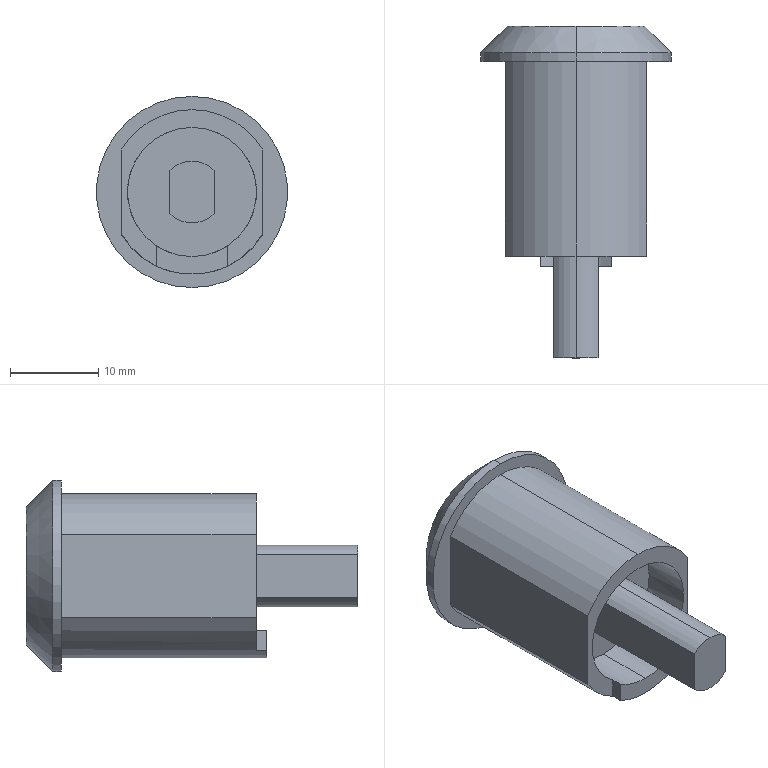Part | SolidWorks | features BaseBody 1 | 1 solid | 36 faces | box 21.6 x 37.5 x 21.6 mm | volume 6258 mm3 | plane 20 | cylinder 14 | cone 2 | commonest cylinder face diameters 7 x5 18.6 x3 10 x2 14.6 x2 21.6 x2
STEP:
#1=CARTESIAN_POINT('',(0.,-33.5,3.5));
#2=VERTEX_POINT('',#1);
#3=CARTESIAN_POINT('',(-2.5,-33.5,2.449));
#4=VERTEX_POINT('',#3);
#5=CARTESIAN_POINT('',(0.,-33.5,0.));
#6=DIRECTION('',(0.,-1.,0.));
#7=DIRECTION('',(0.,0.,1.));
#8=AXIS2_PLACEMENT_3D('',#5,#6,#7);
#9=CIRCLE('',#8,3.5);
#10=EDGE_CURVE('',#2,#4,#9,.T.);
#11=ORIENTED_EDGE('',*,*,#10,.F.);
#12=CARTESIAN_POINT('',(0.,-16.5,3.5));
#13=VERTEX_POINT('',#12);
#14=CARTESIAN_POINT('',(0.,-33.5,3.5));
#15=DIRECTION('',(0.,1.,0.));
#16=VECTOR('',#15,1000.);
#17=LINE('',#14,#16);
#18=EDGE_CURVE('',#2,#13,#17,.T.);
#19=ORIENTED_EDGE('',*,*,#18,.T.);
#20=CARTESIAN_POINT('',(-2.5,-16.5,2.449));
#21=VERTEX_POINT('',#20);
#22=CARTESIAN_POINT('',(0.,-16.5,0.));
#23=DIRECTION('',(0.,1.,0.));
#24=DIRECTION('',(0.,0.,1.));
#25=AXIS2_PLACEMENT_3D('',#22,#23,#24);
#26=CIRCLE('',#25,3.5);
#27=EDGE_CURVE('',#21,#13,#26,.T.);
#28=ORIENTED_EDGE('',*,*,#27,.F.);
#29=CARTESIAN_POINT('',(-2.5,-25.,2.449));
#30=DIRECTION('',(0.,1.,0.));
#31=VECTOR('',#30,1000.);
#32=LINE('',#29,#31);
#33=EDGE_CURVE('',#4,#21,#32,.T.);
#34=ORIENTED_EDGE('',*,*,#33,.F.);
#35=EDGE_LOOP('',(#11,#19,#28,#34));
#36=FACE_OUTER_BOUND('',#35,.T.);
#37=CARTESIAN_POINT('',(0.,-33.5,0.));
#38=DIRECTION('',(0.,1.,0.));
#39=DIRECTION('',(0.,0.,1.));
#40=AXIS2_PLACEMENT_3D('',#37,#38,#39);
#41=CYLINDRICAL_SURFACE('',#40,3.5);
#42=ADVANCED_FACE('',(#36),#41,.T.);
#43=CARTESIAN_POINT('',(0.,-16.5,7.3));
#44=VERTEX_POINT('',#43);
#45=CARTESIAN_POINT('',(0.,-16.5,-7.3));
#46=VERTEX_POINT('',#45);
#47=CARTESIAN_POINT('',(0.,-16.5,0.));
#48=DIRECTION('',(0.,-1.,0.));
#49=DIRECTION('',(0.,0.,-1.));
#50=AXIS2_PLACEMENT_3D('',#47,#48,#49);
#51=CIRCLE('',#50,7.3);
#52=EDGE_CURVE('',#44,#46,#51,.T.);
#53=ORIENTED_EDGE('',*,*,#52,.F.);
#54=CARTESIAN_POINT('',(0.,-22.,7.3));
#55=VERTEX_POINT('',#54);
#56=CARTESIAN_POINT('',(0.,-16.5,7.3));
#57=DIRECTION('',(0.,-1.,0.));
#58=VECTOR('',#57,1000.);
#59=LINE('',#56,#58);
#60=EDGE_CURVE('',#44,#55,#59,.T.);
#61=ORIENTED_EDGE('',*,*,#60,.T.);
#62=CARTESIAN_POINT('',(-4.,-22.,-6.107));
#63=VERTEX_POINT('',#62);
#64=CARTESIAN_POINT('',(0.,-22.,0.));
#65=DIRECTION('',(0.,-1.,0.));
#66=DIRECTION('',(0.,0.,-1.));
#67=AXIS2_PLACEMENT_3D('',#64,#65,#66);
#68=CIRCLE('',#67,7.3);
#69=EDGE_CURVE('',#55,#63,#68,.T.);
#70=ORIENTED_EDGE('',*,*,#69,.T.);
#71=CARTESIAN_POINT('',(-4.,-23.2,-6.107));
#72=VERTEX_POINT('',#71);
#73=CARTESIAN_POINT('',(-4.,-22.6,-6.107));
#74=DIRECTION('',(0.,-1.,0.));
#75=VECTOR('',#74,1000.);
#76=LINE('',#73,#75);
#77=EDGE_CURVE('',#63,#72,#76,.T.);
#78=ORIENTED_EDGE('',*,*,#77,.T.);
#79=CARTESIAN_POINT('',(0.,-23.2,-7.3));
#80=VERTEX_POINT('',#79);
#81=CARTESIAN_POINT('',(0.,-23.2,0.));
#82=DIRECTION('',(0.,-1.,0.));
#83=DIRECTION('',(0.,0.,-1.));
#84=AXIS2_PLACEMENT_3D('',#81,#82,#83);
#85=CIRCLE('',#84,7.3);
#86=EDGE_CURVE('',#72,#80,#85,.T.);
#87=ORIENTED_EDGE('',*,*,#86,.T.);
#88=CARTESIAN_POINT('',(0.,-16.5,-7.3));
#89=DIRECTION('',(0.,-1.,0.));
#90=VECTOR('',#89,1000.);
#91=LINE('',#88,#90);
#92=EDGE_CURVE('',#46,#80,#91,.T.);
#93=ORIENTED_EDGE('',*,*,#92,.F.);
#94=EDGE_LOOP('',(#53,#61,#70,#78,#87,#93));
#95=FACE_OUTER_BOUND('',#94,.T.);
#96=CARTESIAN_POINT('',(0.,-16.5,0.));
#97=DIRECTION('',(0.,-1.,0.));
#98=DIRECTION('',(0.,0.,-1.));
#99=AXIS2_PLACEMENT_3D('',#96,#97,#98);
#100=CYLINDRICAL_SURFACE('',#99,7.3);
#101=ADVANCED_FACE('',(#95),#100,.F.);
#102=CARTESIAN_POINT('',(0.,-22.,9.3));
#103=VERTEX_POINT('',#102);
#104=CARTESIAN_POINT('',(-8.,-22.,4.742));
#105=VERTEX_POINT('',#104);
#106=CARTESIAN_POINT('',(0.,-22.,0.));
#107=DIRECTION('',(0.,-1.,0.));
#108=DIRECTION('',(0.,0.,1.));
#109=AXIS2_PLACEMENT_3D('',#106,#107,#108);
#110=CIRCLE('',#109,9.3);
#111=EDGE_CURVE('',#103,#105,#110,.T.);
#112=ORIENTED_EDGE('',*,*,#111,.F.);
#113=CARTESIAN_POINT('',(0.,0.,9.3));
#114=VERTEX_POINT('',#113);
#115=CARTESIAN_POINT('',(0.,-22.,9.3));
#116=DIRECTION('',(0.,1.,0.));
#117=VECTOR('',#116,1000.);
#118=LINE('',#115,#117);
#119=EDGE_CURVE('',#103,#114,#118,.T.);
#120=ORIENTED_EDGE('',*,*,#119,.T.);
#121=CARTESIAN_POINT('',(-8.,0.,4.742));
#122=VERTEX_POINT('',#121);
#123=CARTESIAN_POINT('',(0.,0.,0.));
#124=DIRECTION('',(0.,1.,0.));
#125=DIRECTION('',(0.,0.,1.));
#126=AXIS2_PLACEMENT_3D('',#123,#124,#125);
#127=CIRCLE('',#126,9.3);
#128=EDGE_CURVE('',#122,#114,#127,.T.);
#129=ORIENTED_EDGE('',*,*,#128,.F.);
#130=CARTESIAN_POINT('',(-8.,-11.,4.742));
#131=DIRECTION('',(0.,-1.,0.));
#132=VECTOR('',#131,1000.);
#133=LINE('',#130,#132);
#134=EDGE_CURVE('',#122,#105,#133,.T.);
#135=ORIENTED_EDGE('',*,*,#134,.T.);
#136=EDGE_LOOP('',(#112,#120,#129,#135));
#137=FACE_OUTER_BOUND('',#136,.T.);
#138=CARTESIAN_POINT('',(0.,-22.,0.));
#139=DIRECTION('',(0.,1.,0.));
#140=DIRECTION('',(0.,0.,1.));
#141=AXIS2_PLACEMENT_3D('',#138,#139,#140);
#142=CYLINDRICAL_SURFACE('',#141,9.3);
#143=ADVANCED_FACE('',(#137),#142,.T.);
#144=CARTESIAN_POINT('',(0.,1.,10.8));
#145=VERTEX_POINT('',#144);
#146=CARTESIAN_POINT('',(0.,1.,-10.8));
#147=VERTEX_POINT('',#146);
#148=CARTESIAN_POINT('',(0.,1.,0.));
#149=DIRECTION('',(0.,1.,0.));
#150=DIRECTION('',(0.,0.,-1.));
#151=AXIS2_PLACEMENT_3D('',#148,#149,#150);
#152=CIRCLE('',#151,10.8);
#153=EDGE_CURVE('',#145,#147,#152,.T.);
#154=ORIENTED_EDGE('',*,*,#153,.F.);
#155=CARTESIAN_POINT('',(0.,0.,10.8));
#156=VERTEX_POINT('',#155);
#157=CARTESIAN_POINT('',(0.,1.,10.8));
#158=DIRECTION('',(0.,-1.,0.));
#159=VECTOR('',#158,1000.);
#160=LINE('',#157,#159);
#161=EDGE_CURVE('',#145,#156,#160,.T.);
#162=ORIENTED_EDGE('',*,*,#161,.T.);
#163=CARTESIAN_POINT('',(0.,0.,-10.8));
#164=VERTEX_POINT('',#163);
#165=CARTESIAN_POINT('',(0.,0.,0.));
#166=DIRECTION('',(0.,1.,0.));
#167=DIRECTION('',(0.,0.,-1.));
#168=AXIS2_PLACEMENT_3D('',#165,#166,#167);
#169=CIRCLE('',#168,10.8);
#170=EDGE_CURVE('',#156,#164,#169,.T.);
#171=ORIENTED_EDGE('',*,*,#170,.T.);
#172=CARTESIAN_POINT('',(0.,1.,-10.8));
#173=DIRECTION('',(0.,-1.,0.));
#174=VECTOR('',#173,1000.);
#175=LINE('',#172,#174);
#176=EDGE_CURVE('',#147,#164,#175,.T.);
#177=ORIENTED_EDGE('',*,*,#176,.F.);
#178=EDGE_LOOP('',(#154,#162,#171,#177));
#179=FACE_OUTER_BOUND('',#178,.T.);
#180=CARTESIAN_POINT('',(0.,1.,0.));
#181=DIRECTION('',(0.,-1.,0.));
#182=DIRECTION('',(0.,0.,-1.));
#183=AXIS2_PLACEMENT_3D('',#180,#181,#182);
#184=CYLINDRICAL_SURFACE('',#183,10.8);
#185=ADVANCED_FACE('',(#179),#184,.T.);
#186=CARTESIAN_POINT('',(0.,4.,7.8));
#187=VERTEX_POINT('',#186);
#188=CARTESIAN_POINT('',(0.,4.,-7.8));
#189=VERTEX_POINT('',#188);
#190=CARTESIAN_POINT('',(0.,4.,0.));
#191=DIRECTION('',(0.,1.,0.));
#192=DIRECTION('',(0.,0.,-1.));
#193=AXIS2_PLACEMENT_3D('',#190,#191,#192);
#194=CIRCLE('',#193,7.8);
#195=EDGE_CURVE('',#187,#189,#194,.T.);
#196=ORIENTED_EDGE('',*,*,#195,.F.);
#197=CARTESIAN_POINT('',(0.,4.,7.8));
#198=DIRECTION('',(0.,-0.7071,0.7071));
#199=VECTOR('',#198,1000.);
#200=LINE('',#197,#199);
#201=EDGE_CURVE('',#187,#145,#200,.T.);
#202=ORIENTED_EDGE('',*,*,#201,.T.);
#203=ORIENTED_EDGE('',*,*,#153,.T.);
#204=CARTESIAN_POINT('',(0.,4.,-7.8));
#205=DIRECTION('',(0.,-0.7071,-0.7071));
#206=VECTOR('',#205,1000.);
#207=LINE('',#204,#206);
#208=EDGE_CURVE('',#189,#147,#207,.T.);
#209=ORIENTED_EDGE('',*,*,#208,.F.);
#210=EDGE_LOOP('',(#196,#202,#203,#209));
#211=FACE_OUTER_BOUND('',#210,.T.);
#212=CARTESIAN_POINT('',(0.,4.,0.));
#213=DIRECTION('',(0.,-1.,0.));
#214=DIRECTION('',(0.,0.,-1.));
#215=AXIS2_PLACEMENT_3D('',#212,#213,#214);
#216=CONICAL_SURFACE('',#215,7.8,0.7854);
#217=ADVANCED_FACE('',(#211),#216,.T.);
#218=CARTESIAN_POINT('',(0.,4.,-5.));
#219=VERTEX_POINT('',#218);
#220=CARTESIAN_POINT('',(1.,4.,4.899));
#221=VERTEX_POINT('',#220);
#222=CARTESIAN_POINT('',(0.,4.,0.));
#223=DIRECTION('',(0.,-1.,0.));
#224=DIRECTION('',(0.,0.,-1.));
#225=AXIS2_PLACEMENT_3D('',#222,#223,#224);
#226=CIRCLE('',#225,5.);
#227=EDGE_CURVE('',#219,#221,#226,.T.);
#228=ORIENTED_EDGE('',*,*,#227,.F.);
#229=CARTESIAN_POINT('',(0.,0.,-5.));
#230=VERTEX_POINT('',#229);
#231=CARTESIAN_POINT('',(0.,4.,-5.));
#232=DIRECTION('',(0.,-1.,0.));
#233=VECTOR('',#232,1000.);
#234=LINE('',#231,#233);
#235=EDGE_CURVE('',#219,#230,#234,.T.);
#236=ORIENTED_EDGE('',*,*,#235,.T.);
#237=CARTESIAN_POINT('',(1.,0.,4.899));
#238=VERTEX_POINT('',#237);
#239=CARTESIAN_POINT('',(0.,0.,0.));
#240=DIRECTION('',(0.,-1.,0.));
#241=DIRECTION('',(0.,0.,-1.));
#242=AXIS2_PLACEMENT_3D('',#239,#240,#241);
#243=CIRCLE('',#242,5.);
#244=EDGE_CURVE('',#230,#238,#243,.T.);
#245=ORIENTED_EDGE('',*,*,#244,.T.);
#246=CARTESIAN_POINT('',(1.,2.,4.899));
#247=DIRECTION('',(0.,1.,0.));
#248=VECTOR('',#247,1000.);
#249=LINE('',#246,#248);
#250=EDGE_CURVE('',#238,#221,#249,.T.);
#251=ORIENTED_EDGE('',*,*,#250,.T.);
#252=EDGE_LOOP('',(#228,#236,#245,#251));
#253=FACE_OUTER_BOUND('',#252,.T.);
#254=CARTESIAN_POINT('',(0.,4.,0.));
#255=DIRECTION('',(0.,-1.,0.));
#256=DIRECTION('',(0.,0.,-1.));
#257=AXIS2_PLACEMENT_3D('',#254,#255,#256);
#258=CYLINDRICAL_SURFACE('',#257,5.);
#259=ADVANCED_FACE('',(#253),#258,.F.);
#260=CARTESIAN_POINT('',(0.,4.,-3.5));
#261=VERTEX_POINT('',#260);
#262=CARTESIAN_POINT('',(-1.,4.,3.354));
#263=VERTEX_POINT('',#262);
#264=CARTESIAN_POINT('',(0.,4.,0.));
#265=DIRECTION('',(0.,1.,0.));
#266=DIRECTION('',(0.,0.,-1.));
#267=AXIS2_PLACEMENT_3D('',#264,#265,#266);
#268=CIRCLE('',#267,3.5);
#269=EDGE_CURVE('',#261,#263,#268,.T.);
#270=ORIENTED_EDGE('',*,*,#269,.F.);
#271=CARTESIAN_POINT('',(0.,0.,-3.5));
#272=VERTEX_POINT('',#271);
#273=CARTESIAN_POINT('',(0.,4.,-3.5));
#274=DIRECTION('',(0.,-1.,0.));
#275=VECTOR('',#274,1000.);
#276=LINE('',#273,#275);
#277=EDGE_CURVE('',#261,#272,#276,.T.);
#278=ORIENTED_EDGE('',*,*,#277,.T.);
#279=CARTESIAN_POINT('',(-1.,0.,3.354));
#280=VERTEX_POINT('',#279);
#281=CARTESIAN_POINT('',(0.,0.,0.));
#282=DIRECTION('',(0.,1.,0.));
#283=DIRECTION('',(0.,0.,-1.));
#284=AXIS2_PLACEMENT_3D('',#281,#282,#283);
#285=CIRCLE('',#284,3.5);
#286=EDGE_CURVE('',#272,#280,#285,.T.);
#287=ORIENTED_EDGE('',*,*,#286,.T.);
#288=CARTESIAN_POINT('',(-1.,2.,3.354));
#289=DIRECTION('',(0.,-1.,0.));
#290=VECTOR('',#289,1000.);
#291=LINE('',#288,#290);
#292=EDGE_CURVE('',#263,#280,#291,.T.);
#293=ORIENTED_EDGE('',*,*,#292,.F.);
#294=EDGE_LOOP('',(#270,#278,#287,#293));
#295=FACE_OUTER_BOUND('',#294,.T.);
#296=CARTESIAN_POINT('',(0.,4.,0.));
#297=DIRECTION('',(0.,-1.,0.));
#298=DIRECTION('',(0.,0.,-1.));
#299=AXIS2_PLACEMENT_3D('',#296,#297,#298);
#300=CYLINDRICAL_SURFACE('',#299,3.5);
#301=ADVANCED_FACE('',(#295),#300,.T.);
#302=ORIENTED_EDGE('',*,*,#18,.F.);
#303=CARTESIAN_POINT('',(2.5,-33.5,2.449));
#304=VERTEX_POINT('',#303);
#305=CARTESIAN_POINT('',(0.,-33.5,0.));
#306=DIRECTION('',(0.,-1.,0.));
#307=DIRECTION('',(0.,0.,1.));
#308=AXIS2_PLACEMENT_3D('',#305,#306,#307);
#309=CIRCLE('',#308,3.5);
#310=EDGE_CURVE('',#304,#2,#309,.T.);
#311=ORIENTED_EDGE('',*,*,#310,.F.);
#312=CARTESIAN_POINT('',(2.5,-16.5,2.449));
#313=VERTEX_POINT('',#312);
#314=CARTESIAN_POINT('',(2.5,-25.,2.449));
#315=DIRECTION('',(0.,-1.,0.));
#316=VECTOR('',#315,1000.);
#317=LINE('',#314,#316);
#318=EDGE_CURVE('',#313,#304,#317,.T.);
#319=ORIENTED_EDGE('',*,*,#318,.F.);
#320=CARTESIAN_POINT('',(0.,-16.5,0.));
#321=DIRECTION('',(0.,1.,0.));
#322=DIRECTION('',(0.,0.,1.));
#323=AXIS2_PLACEMENT_3D('',#320,#321,#322);
#324=CIRCLE('',#323,3.5);
#325=EDGE_CURVE('',#13,#313,#324,.T.);
#326=ORIENTED_EDGE('',*,*,#325,.F.);
#327=EDGE_LOOP('',(#302,#311,#319,#326));
#328=FACE_OUTER_BOUND('',#327,.T.);
#329=CARTESIAN_POINT('',(0.,-33.5,0.));
#330=DIRECTION('',(0.,1.,0.));
#331=DIRECTION('',(0.,0.,1.));
#332=AXIS2_PLACEMENT_3D('',#329,#330,#331);
#333=CYLINDRICAL_SURFACE('',#332,3.5);
#334=ADVANCED_FACE('',(#328),#333,.T.);
#335=ORIENTED_EDGE('',*,*,#310,.T.);
#336=ORIENTED_EDGE('',*,*,#10,.T.);
#337=CARTESIAN_POINT('',(-2.5,-33.5,-2.449));
#338=VERTEX_POINT('',#337);
#339=CARTESIAN_POINT('',(-2.5,-33.5,0.));
#340=DIRECTION('',(0.,0.,-1.));
#341=VECTOR('',#340,1000.);
#342=LINE('',#339,#341);
#343=EDGE_CURVE('',#4,#338,#342,.T.);
#344=ORIENTED_EDGE('',*,*,#343,.T.);
#345=CARTESIAN_POINT('',(2.5,-33.5,-2.449));
#346=VERTEX_POINT('',#345);
#347=CARTESIAN_POINT('',(0.,-33.5,0.));
#348=DIRECTION('',(0.,-1.,0.));
#349=DIRECTION('',(0.,0.,1.));
#350=AXIS2_PLACEMENT_3D('',#347,#348,#349);
#351=CIRCLE('',#350,3.5);
#352=EDGE_CURVE('',#338,#346,#351,.T.);
#353=ORIENTED_EDGE('',*,*,#352,.T.);
#354=CARTESIAN_POINT('',(2.5,-33.5,0.));
#355=DIRECTION('',(0.,0.,1.));
#356=VECTOR('',#355,1000.);
#357=LINE('',#354,#356);
#358=EDGE_CURVE('',#346,#304,#357,.T.);
#359=ORIENTED_EDGE('',*,*,#358,.T.);
#360=EDGE_LOOP('',(#335,#336,#344,#353,#359));
#361=FACE_OUTER_BOUND('',#360,.T.);
#362=CARTESIAN_POINT('',(-2.5,-33.5,3.542));
#363=DIRECTION('',(0.,-1.,0.));
#364=DIRECTION('',(0.,0.,-1.));
#365=AXIS2_PLACEMENT_3D('',#362,#363,#364);
#366=PLANE('',#365);
#367=ADVANCED_FACE('',(#361),#366,.T.);
#368=ORIENTED_EDGE('',*,*,#27,.T.);
#369=ORIENTED_EDGE('',*,*,#325,.T.);
#370=CARTESIAN_POINT('',(2.5,-16.5,-2.449));
#371=VERTEX_POINT('',#370);
#372=CARTESIAN_POINT('',(2.5,-16.5,0.));
#373=DIRECTION('',(0.,0.,-1.));
#374=VECTOR('',#373,1000.);
#375=LINE('',#372,#374);
#376=EDGE_CURVE('',#313,#371,#375,.T.);
#377=ORIENTED_EDGE('',*,*,#376,.T.);
#378=CARTESIAN_POINT('',(-2.5,-16.5,-2.449));
#379=VERTEX_POINT('',#378);
#380=CARTESIAN_POINT('',(0.,-16.5,0.));
#381=DIRECTION('',(0.,1.,0.));
#382=DIRECTION('',(0.,0.,1.));
#383=AXIS2_PLACEMENT_3D('',#380,#381,#382);
#384=CIRCLE('',#383,3.5);
#385=EDGE_CURVE('',#371,#379,#384,.T.);
#386=ORIENTED_EDGE('',*,*,#385,.T.);
#387=CARTESIAN_POINT('',(-2.5,-16.5,0.));
#388=DIRECTION('',(0.,0.,1.));
#389=VECTOR('',#388,1000.);
#390=LINE('',#387,#389);
#391=EDGE_CURVE('',#379,#21,#390,.T.);
#392=ORIENTED_EDGE('',*,*,#391,.T.);
#393=EDGE_LOOP('',(#368,#369,#377,#386,#392));
#394=FACE_BOUND('',#393,.T.);
#395=CARTESIAN_POINT('',(0.,-16.5,0.));
#396=DIRECTION('',(0.,-1.,0.));
#397=DIRECTION('',(0.,0.,-1.));
#398=AXIS2_PLACEMENT_3D('',#395,#396,#397);
#399=CIRCLE('',#398,7.3);
#400=EDGE_CURVE('',#46,#44,#399,.T.);
#401=ORIENTED_EDGE('',*,*,#400,.T.);
#402=ORIENTED_EDGE('',*,*,#52,.T.);
#403=EDGE_LOOP('',(#401,#402));
#404=FACE_OUTER_BOUND('',#403,.T.);
#405=CARTESIAN_POINT('',(-7.388,-16.5,7.388));
#406=DIRECTION('',(0.,-1.,0.));
#407=DIRECTION('',(0.,0.,-1.));
#408=AXIS2_PLACEMENT_3D('',#405,#406,#407);
#409=PLANE('',#408);
#410=ADVANCED_FACE('',(#394,#404),#409,.T.);
#411=CARTESIAN_POINT('',(-2.5,-25.,-2.449));
#412=DIRECTION('',(0.,1.,0.));
#413=VECTOR('',#412,1000.);
#414=LINE('',#411,#413);
#415=EDGE_CURVE('',#338,#379,#414,.T.);
#416=ORIENTED_EDGE('',*,*,#415,.F.);
#417=ORIENTED_EDGE('',*,*,#343,.F.);
#418=ORIENTED_EDGE('',*,*,#33,.T.);
#419=ORIENTED_EDGE('',*,*,#391,.F.);
#420=EDGE_LOOP('',(#416,#417,#418,#419));
#421=FACE_OUTER_BOUND('',#420,.T.);
#422=CARTESIAN_POINT('',(-2.5,-33.5,2.449));
#423=DIRECTION('',(1.,0.,0.));
#424=DIRECTION('',(0.,0.,-1.));
#425=AXIS2_PLACEMENT_3D('',#422,#423,#424);
#426=PLANE('',#425);
#427=ADVANCED_FACE('',(#421),#426,.F.);
#428=ORIENTED_EDGE('',*,*,#318,.T.);
#429=ORIENTED_EDGE('',*,*,#358,.F.);
#430=CARTESIAN_POINT('',(2.5,-25.,-2.449));
#431=DIRECTION('',(0.,-1.,0.));
#432=VECTOR('',#431,1000.);
#433=LINE('',#430,#432);
#434=EDGE_CURVE('',#371,#346,#433,.T.);
#435=ORIENTED_EDGE('',*,*,#434,.F.);
#436=ORIENTED_EDGE('',*,*,#376,.F.);
#437=EDGE_LOOP('',(#428,#429,#435,#436));
#438=FACE_OUTER_BOUND('',#437,.T.);
#439=CARTESIAN_POINT('',(2.5,-33.5,-2.449));
#440=DIRECTION('',(-1.,0.,0.));
#441=DIRECTION('',(0.,0.,1.));
#442=AXIS2_PLACEMENT_3D('',#439,#440,#441);
#443=PLANE('',#442);
#444=ADVANCED_FACE('',(#438),#443,.F.);
#445=ORIENTED_EDGE('',*,*,#434,.T.);
#446=ORIENTED_EDGE('',*,*,#352,.F.);
#447=ORIENTED_EDGE('',*,*,#415,.T.);
#448=ORIENTED_EDGE('',*,*,#385,.F.);
#449=EDGE_LOOP('',(#445,#446,#447,#448));
#450=FACE_OUTER_BOUND('',#449,.T.);
#451=CARTESIAN_POINT('',(0.,-33.5,0.));
#452=DIRECTION('',(0.,1.,0.));
#453=DIRECTION('',(0.,0.,1.));
#454=AXIS2_PLACEMENT_3D('',#451,#452,#453);
#455=CYLINDRICAL_SURFACE('',#454,3.5);
#456=ADVANCED_FACE('',(#450),#455,.T.);
#457=ORIENTED_EDGE('',*,*,#60,.F.);
#458=ORIENTED_EDGE('',*,*,#400,.F.);
#459=ORIENTED_EDGE('',*,*,#92,.T.);
#460=CARTESIAN_POINT('',(4.,-23.2,-6.107));
#461=VERTEX_POINT('',#460);
#462=CARTESIAN_POINT('',(0.,-23.2,0.));
#463=DIRECTION('',(0.,-1.,0.));
#464=DIRECTION('',(0.,0.,-1.));
#465=AXIS2_PLACEMENT_3D('',#462,#463,#464);
#466=CIRCLE('',#465,7.3);
#467=EDGE_CURVE('',#80,#461,#466,.T.);
#468=ORIENTED_EDGE('',*,*,#467,.T.);
#469=CARTESIAN_POINT('',(4.,-22.,-6.107));
#470=VERTEX_POINT('',#469);
#471=CARTESIAN_POINT('',(4.,-22.6,-6.107));
#472=DIRECTION('',(0.,1.,0.));
#473=VECTOR('',#472,1000.);
#474=LINE('',#471,#473);
#475=EDGE_CURVE('',#461,#470,#474,.T.);
#476=ORIENTED_EDGE('',*,*,#475,.T.);
#477=CARTESIAN_POINT('',(0.,-22.,0.));
#478=DIRECTION('',(0.,-1.,0.));
#479=DIRECTION('',(0.,0.,-1.));
#480=AXIS2_PLACEMENT_3D('',#477,#478,#479);
#481=CIRCLE('',#480,7.3);
#482=EDGE_CURVE('',#470,#55,#481,.T.);
#483=ORIENTED_EDGE('',*,*,#482,.T.);
#484=EDGE_LOOP('',(#457,#458,#459,#468,#476,#483));
#485=FACE_OUTER_BOUND('',#484,.T.);
#486=CARTESIAN_POINT('',(0.,-16.5,0.));
#487=DIRECTION('',(0.,-1.,0.));
#488=DIRECTION('',(0.,0.,-1.));
#489=AXIS2_PLACEMENT_3D('',#486,#487,#488);
#490=CYLINDRICAL_SURFACE('',#489,7.3);
#491=ADVANCED_FACE('',(#485),#490,.F.);
#492=ORIENTED_EDGE('',*,*,#86,.F.);
#493=CARTESIAN_POINT('',(-4.,-23.2,-8.396));
#494=VERTEX_POINT('',#493);
#495=CARTESIAN_POINT('',(-4.,-23.2,-7.703));
#496=DIRECTION('',(0.,0.,-1.));
#497=VECTOR('',#496,1000.);
#498=LINE('',#495,#497);
#499=EDGE_CURVE('',#72,#494,#498,.T.);
#500=ORIENTED_EDGE('',*,*,#499,.T.);
#501=CARTESIAN_POINT('',(4.,-23.2,-8.396));
#502=VERTEX_POINT('',#501);
#503=CARTESIAN_POINT('',(0.,-23.2,0.));
#504=DIRECTION('',(0.,-1.,0.));
#505=DIRECTION('',(0.,0.,1.));
#506=AXIS2_PLACEMENT_3D('',#503,#504,#505);
#507=CIRCLE('',#506,9.3);
#508=EDGE_CURVE('',#494,#502,#507,.T.);
#509=ORIENTED_EDGE('',*,*,#508,.T.);
#510=CARTESIAN_POINT('',(4.,-23.2,-7.703));
#511=DIRECTION('',(0.,0.,1.));
#512=VECTOR('',#511,1000.);
#513=LINE('',#510,#512);
#514=EDGE_CURVE('',#502,#461,#513,.T.);
#515=ORIENTED_EDGE('',*,*,#514,.T.);
#516=ORIENTED_EDGE('',*,*,#467,.F.);
#517=EDGE_LOOP('',(#492,#500,#509,#515,#516));
#518=FACE_OUTER_BOUND('',#517,.T.);
#519=CARTESIAN_POINT('',(-4.,-23.2,-6.087));
#520=DIRECTION('',(0.,-1.,0.));
#521=DIRECTION('',(0.,0.,-1.));
#522=AXIS2_PLACEMENT_3D('',#519,#520,#521);
#523=PLANE('',#522);
#524=ADVANCED_FACE('',(#518),#523,.T.);
#525=CARTESIAN_POINT('',(-8.,-22.,-4.742));
#526=VERTEX_POINT('',#525);
#527=CARTESIAN_POINT('',(-8.,-22.,0.4521));
#528=DIRECTION('',(0.,0.,-1.));
#529=VECTOR('',#528,1000.);
#530=LINE('',#527,#529);
#531=EDGE_CURVE('',#105,#526,#530,.T.);
#532=ORIENTED_EDGE('',*,*,#531,.T.);
#533=CARTESIAN_POINT('',(-4.,-22.,-8.396));
#534=VERTEX_POINT('',#533);
#535=CARTESIAN_POINT('',(0.,-22.,0.));
#536=DIRECTION('',(0.,-1.,0.));
#537=DIRECTION('',(0.,0.,1.));
#538=AXIS2_PLACEMENT_3D('',#535,#536,#537);
#539=CIRCLE('',#538,9.3);
#540=EDGE_CURVE('',#526,#534,#539,.T.);
#541=ORIENTED_EDGE('',*,*,#540,.T.);
#542=CARTESIAN_POINT('',(-4.,-22.,0.4521));
#543=DIRECTION('',(0.,0.,1.));
#544=VECTOR('',#543,1000.);
#545=LINE('',#542,#544);
#546=EDGE_CURVE('',#534,#63,#545,.T.);
#547=ORIENTED_EDGE('',*,*,#546,.T.);
#548=ORIENTED_EDGE('',*,*,#69,.F.);
#549=ORIENTED_EDGE('',*,*,#482,.F.);
#550=CARTESIAN_POINT('',(4.,-22.,-8.396));
#551=VERTEX_POINT('',#550);
#552=CARTESIAN_POINT('',(4.,-22.,0.4521));
#553=DIRECTION('',(0.,0.,-1.));
#554=VECTOR('',#553,1000.);
#555=LINE('',#552,#554);
#556=EDGE_CURVE('',#470,#551,#555,.T.);
#557=ORIENTED_EDGE('',*,*,#556,.T.);
#558=CARTESIAN_POINT('',(8.,-22.,-4.742));
#559=VERTEX_POINT('',#558);
#560=CARTESIAN_POINT('',(0.,-22.,0.));
#561=DIRECTION('',(0.,-1.,0.));
#562=DIRECTION('',(0.,0.,1.));
#563=AXIS2_PLACEMENT_3D('',#560,#561,#562);
#564=CIRCLE('',#563,9.3);
#565=EDGE_CURVE('',#551,#559,#564,.T.);
#566=ORIENTED_EDGE('',*,*,#565,.T.);
#567=CARTESIAN_POINT('',(8.,-22.,4.742));
#568=VERTEX_POINT('',#567);
#569=CARTESIAN_POINT('',(8.,-22.,0.4521));
#570=DIRECTION('',(0.,0.,1.));
#571=VECTOR('',#570,1000.);
#572=LINE('',#569,#571);
#573=EDGE_CURVE('',#559,#568,#572,.T.);
#574=ORIENTED_EDGE('',*,*,#573,.T.);
#575=CARTESIAN_POINT('',(0.,-22.,0.));
#576=DIRECTION('',(0.,-1.,0.));
#577=DIRECTION('',(0.,0.,1.));
#578=AXIS2_PLACEMENT_3D('',#575,#576,#577);
#579=CIRCLE('',#578,9.3);
#580=EDGE_CURVE('',#568,#103,#579,.T.);
#581=ORIENTED_EDGE('',*,*,#580,.T.);
#582=ORIENTED_EDGE('',*,*,#111,.T.);
#583=EDGE_LOOP('',(#532,#541,#547,#548,#549,#557,#566,#574,#581,#582));
#584=FACE_OUTER_BOUND('',#583,.T.);
#585=CARTESIAN_POINT('',(-8.,-22.,9.406));
#586=DIRECTION('',(0.,-1.,0.));
#587=DIRECTION('',(0.,0.,-1.));
#588=AXIS2_PLACEMENT_3D('',#585,#586,#587);
#589=PLANE('',#588);
#590=ADVANCED_FACE('',(#584),#589,.T.);
#591=CARTESIAN_POINT('',(-4.,-22.6,-8.396));
#592=DIRECTION('',(0.,1.,0.));
#593=VECTOR('',#592,1000.);
#594=LINE('',#591,#593);
#595=EDGE_CURVE('',#494,#534,#594,.T.);
#596=ORIENTED_EDGE('',*,*,#595,.F.);
#597=ORIENTED_EDGE('',*,*,#499,.F.);
#598=ORIENTED_EDGE('',*,*,#77,.F.);
#599=ORIENTED_EDGE('',*,*,#546,.F.);
#600=EDGE_LOOP('',(#596,#597,#598,#599));
#601=FACE_OUTER_BOUND('',#600,.T.);
#602=CARTESIAN_POINT('',(-4.,-23.2,-6.107));
#603=DIRECTION('',(1.,0.,0.));
#604=DIRECTION('',(0.,0.,-1.));
#605=AXIS2_PLACEMENT_3D('',#602,#603,#604);
#606=PLANE('',#605);
#607=ADVANCED_FACE('',(#601),#606,.F.);
#608=ORIENTED_EDGE('',*,*,#475,.F.);
#609=ORIENTED_EDGE('',*,*,#514,.F.);
#610=CARTESIAN_POINT('',(4.,-22.6,-8.396));
#611=DIRECTION('',(0.,-1.,0.));
#612=VECTOR('',#611,1000.);
#613=LINE('',#610,#612);
#614=EDGE_CURVE('',#551,#502,#613,.T.);
#615=ORIENTED_EDGE('',*,*,#614,.F.);
#616=ORIENTED_EDGE('',*,*,#556,.F.);
#617=EDGE_LOOP('',(#608,#609,#615,#616));
#618=FACE_OUTER_BOUND('',#617,.T.);
#619=CARTESIAN_POINT('',(4.,-23.2,-8.396));
#620=DIRECTION('',(-1.,0.,0.));
#621=DIRECTION('',(0.,0.,1.));
#622=AXIS2_PLACEMENT_3D('',#619,#620,#621);
#623=PLANE('',#622);
#624=ADVANCED_FACE('',(#618),#623,.F.);
#625=CARTESIAN_POINT('',(8.,0.,-4.742));
#626=VERTEX_POINT('',#625);
#627=CARTESIAN_POINT('',(8.,-11.6,-4.742));
#628=DIRECTION('',(0.,1.,0.));
#629=VECTOR('',#628,1000.);
#630=LINE('',#627,#629);
#631=EDGE_CURVE('',#559,#626,#630,.T.);
#632=ORIENTED_EDGE('',*,*,#631,.F.);
#633=ORIENTED_EDGE('',*,*,#565,.F.);
#634=ORIENTED_EDGE('',*,*,#614,.T.);
#635=ORIENTED_EDGE('',*,*,#508,.F.);
#636=ORIENTED_EDGE('',*,*,#595,.T.);
#637=ORIENTED_EDGE('',*,*,#540,.F.);
#638=CARTESIAN_POINT('',(-8.,0.,-4.742));
#639=VERTEX_POINT('',#638);
#640=CARTESIAN_POINT('',(-8.,-11.6,-4.742));
#641=DIRECTION('',(0.,-1.,0.));
#642=VECTOR('',#641,1000.);
#643=LINE('',#640,#642);
#644=EDGE_CURVE('',#639,#526,#643,.T.);
#645=ORIENTED_EDGE('',*,*,#644,.F.);
#646=CARTESIAN_POINT('',(0.,0.,0.));
#647=DIRECTION('',(0.,1.,0.));
#648=DIRECTION('',(0.,0.,1.));
#649=AXIS2_PLACEMENT_3D('',#646,#647,#648);
#650=CIRCLE('',#649,9.3);
#651=EDGE_CURVE('',#626,#639,#650,.T.);
#652=ORIENTED_EDGE('',*,*,#651,.F.);
#653=EDGE_LOOP('',(#632,#633,#634,#635,#636,#637,#645,#652));
#654=FACE_OUTER_BOUND('',#653,.T.);
#655=CARTESIAN_POINT('',(0.,-23.2,0.));
#656=DIRECTION('',(0.,1.,0.));
#657=DIRECTION('',(0.,0.,1.));
#658=AXIS2_PLACEMENT_3D('',#655,#656,#657);
#659=CYLINDRICAL_SURFACE('',#658,9.3);
#660=ADVANCED_FACE('',(#654),#659,.T.);
#661=ORIENTED_EDGE('',*,*,#644,.T.);
#662=ORIENTED_EDGE('',*,*,#531,.F.);
#663=ORIENTED_EDGE('',*,*,#134,.F.);
#664=CARTESIAN_POINT('',(-8.,0.,0.));
#665=DIRECTION('',(0.,0.,1.));
#666=VECTOR('',#665,1000.);
#667=LINE('',#664,#666);
#668=EDGE_CURVE('',#639,#122,#667,.T.);
#669=ORIENTED_EDGE('',*,*,#668,.F.);
#670=EDGE_LOOP('',(#661,#662,#663,#669));
#671=FACE_OUTER_BOUND('',#670,.T.);
#672=CARTESIAN_POINT('',(-8.,-22.,4.742));
#673=DIRECTION('',(1.,0.,0.));
#674=DIRECTION('',(0.,0.,-1.));
#675=AXIS2_PLACEMENT_3D('',#672,#673,#674);
#676=PLANE('',#675);
#677=ADVANCED_FACE('',(#671),#676,.F.);
#678=ORIENTED_EDGE('',*,*,#119,.F.);
#679=ORIENTED_EDGE('',*,*,#580,.F.);
#680=CARTESIAN_POINT('',(8.,0.,4.742));
#681=VERTEX_POINT('',#680);
#682=CARTESIAN_POINT('',(8.,-11.,4.742));
#683=DIRECTION('',(0.,-1.,0.));
#684=VECTOR('',#683,1000.);
#685=LINE('',#682,#684);
#686=EDGE_CURVE('',#681,#568,#685,.T.);
#687=ORIENTED_EDGE('',*,*,#686,.F.);
#688=CARTESIAN_POINT('',(0.,0.,0.));
#689=DIRECTION('',(0.,1.,0.));
#690=DIRECTION('',(0.,0.,1.));
#691=AXIS2_PLACEMENT_3D('',#688,#689,#690);
#692=CIRCLE('',#691,9.3);
#693=EDGE_CURVE('',#114,#681,#692,.T.);
#694=ORIENTED_EDGE('',*,*,#693,.F.);
#695=EDGE_LOOP('',(#678,#679,#687,#694));
#696=FACE_OUTER_BOUND('',#695,.T.);
#697=CARTESIAN_POINT('',(0.,-22.,0.));
#698=DIRECTION('',(0.,1.,0.));
#699=DIRECTION('',(0.,0.,1.));
#700=AXIS2_PLACEMENT_3D('',#697,#698,#699);
#701=CYLINDRICAL_SURFACE('',#700,9.3);
#702=ADVANCED_FACE('',(#696),#701,.T.);
#703=ORIENTED_EDGE('',*,*,#686,.T.);
#704=ORIENTED_EDGE('',*,*,#573,.F.);
#705=ORIENTED_EDGE('',*,*,#631,.T.);
#706=CARTESIAN_POINT('',(8.,0.,0.));
#707=DIRECTION('',(0.,0.,-1.));
#708=VECTOR('',#707,1000.);
#709=LINE('',#706,#708);
#710=EDGE_CURVE('',#681,#626,#709,.T.);
#711=ORIENTED_EDGE('',*,*,#710,.F.);
#712=EDGE_LOOP('',(#703,#704,#705,#711));
#713=FACE_OUTER_BOUND('',#712,.T.);
#714=CARTESIAN_POINT('',(8.,-22.,-4.742));
#715=DIRECTION('',(-1.,0.,0.));
#716=DIRECTION('',(0.,0.,1.));
#717=AXIS2_PLACEMENT_3D('',#714,#715,#716);
#718=PLANE('',#717);
#719=ADVANCED_FACE('',(#713),#718,.F.);
#720=ORIENTED_EDGE('',*,*,#668,.T.);
#721=ORIENTED_EDGE('',*,*,#128,.T.);
#722=ORIENTED_EDGE('',*,*,#693,.T.);
#723=ORIENTED_EDGE('',*,*,#710,.T.);
#724=ORIENTED_EDGE('',*,*,#651,.T.);
#725=EDGE_LOOP('',(#720,#721,#722,#723,#724));
#726=FACE_BOUND('',#725,.T.);
#727=CARTESIAN_POINT('',(0.,0.,0.));
#728=DIRECTION('',(0.,1.,0.));
#729=DIRECTION('',(0.,0.,-1.));
#730=AXIS2_PLACEMENT_3D('',#727,#728,#729);
#731=CIRCLE('',#730,10.8);
#732=EDGE_CURVE('',#164,#156,#731,.T.);
#733=ORIENTED_EDGE('',*,*,#732,.F.);
#734=ORIENTED_EDGE('',*,*,#170,.F.);
#735=EDGE_LOOP('',(#733,#734));
#736=FACE_OUTER_BOUND('',#735,.T.);
#737=CARTESIAN_POINT('',(-10.93,0.,-10.93));
#738=DIRECTION('',(0.,1.,0.));
#739=DIRECTION('',(0.,0.,1.));
#740=AXIS2_PLACEMENT_3D('',#737,#738,#739);
#741=PLANE('',#740);
#742=ADVANCED_FACE('',(#726,#736),#741,.F.);
#743=ORIENTED_EDGE('',*,*,#161,.F.);
#744=CARTESIAN_POINT('',(0.,1.,0.));
#745=DIRECTION('',(0.,1.,0.));
#746=DIRECTION('',(0.,0.,-1.));
#747=AXIS2_PLACEMENT_3D('',#744,#745,#746);
#748=CIRCLE('',#747,10.8);
#749=EDGE_CURVE('',#147,#145,#748,.T.);
#750=ORIENTED_EDGE('',*,*,#749,.F.);
#751=ORIENTED_EDGE('',*,*,#176,.T.);
#752=ORIENTED_EDGE('',*,*,#732,.T.);
#753=EDGE_LOOP('',(#743,#750,#751,#752));
#754=FACE_OUTER_BOUND('',#753,.T.);
#755=CARTESIAN_POINT('',(0.,1.,0.));
#756=DIRECTION('',(0.,-1.,0.));
#757=DIRECTION('',(0.,0.,-1.));
#758=AXIS2_PLACEMENT_3D('',#755,#756,#757);
#759=CYLINDRICAL_SURFACE('',#758,10.8);
#760=ADVANCED_FACE('',(#754),#759,.T.);
#761=ORIENTED_EDGE('',*,*,#201,.F.);
#762=CARTESIAN_POINT('',(0.,4.,0.));
#763=DIRECTION('',(0.,1.,0.));
#764=DIRECTION('',(0.,0.,-1.));
#765=AXIS2_PLACEMENT_3D('',#762,#763,#764);
#766=CIRCLE('',#765,7.8);
#767=EDGE_CURVE('',#189,#187,#766,.T.);
#768=ORIENTED_EDGE('',*,*,#767,.F.);
#769=ORIENTED_EDGE('',*,*,#208,.T.);
#770=ORIENTED_EDGE('',*,*,#749,.T.);
#771=EDGE_LOOP('',(#761,#768,#769,#770));
#772=FACE_OUTER_BOUND('',#771,.T.);
#773=CARTESIAN_POINT('',(0.,4.,0.));
#774=DIRECTION('',(0.,-1.,0.));
#775=DIRECTION('',(0.,0.,-1.));
#776=AXIS2_PLACEMENT_3D('',#773,#774,#775);
#777=CONICAL_SURFACE('',#776,7.8,0.7854);
#778=ADVANCED_FACE('',(#772),#777,.T.);
#779=CARTESIAN_POINT('',(-1.,4.,4.899));
#780=VERTEX_POINT('',#779);
#781=CARTESIAN_POINT('',(-1.,4.,6.25));
#782=VERTEX_POINT('',#781);
#783=CARTESIAN_POINT('',(-1.,4.,5.574));
#784=DIRECTION('',(0.,0.,1.));
#785=VECTOR('',#784,1000.);
#786=LINE('',#783,#785);
#787=EDGE_CURVE('',#780,#782,#786,.T.);
#788=ORIENTED_EDGE('',*,*,#787,.F.);
#789=CARTESIAN_POINT('',(0.,4.,0.));
#790=DIRECTION('',(0.,-1.,0.));
#791=DIRECTION('',(0.,0.,-1.));
#792=AXIS2_PLACEMENT_3D('',#789,#790,#791);
#793=CIRCLE('',#792,5.);
#794=EDGE_CURVE('',#780,#219,#793,.T.);
#795=ORIENTED_EDGE('',*,*,#794,.T.);
#796=ORIENTED_EDGE('',*,*,#227,.T.);
#797=CARTESIAN_POINT('',(1.,4.,6.25));
#798=VERTEX_POINT('',#797);
#799=CARTESIAN_POINT('',(1.,4.,5.574));
#800=DIRECTION('',(0.,0.,1.));
#801=VECTOR('',#800,1000.);
#802=LINE('',#799,#801);
#803=EDGE_CURVE('',#221,#798,#802,.T.);
#804=ORIENTED_EDGE('',*,*,#803,.T.);
#805=CARTESIAN_POINT('',(0.,4.,6.25));
#806=DIRECTION('',(-1.,0.,0.));
#807=VECTOR('',#806,1000.);
#808=LINE('',#805,#807);
#809=EDGE_CURVE('',#798,#782,#808,.T.);
#810=ORIENTED_EDGE('',*,*,#809,.T.);
#811=EDGE_LOOP('',(#788,#795,#796,#804,#810));
#812=FACE_BOUND('',#811,.T.);
#813=ORIENTED_EDGE('',*,*,#767,.T.);
#814=ORIENTED_EDGE('',*,*,#195,.T.);
#815=EDGE_LOOP('',(#813,#814));
#816=FACE_OUTER_BOUND('',#815,.T.);
#817=CARTESIAN_POINT('',(-7.894,4.,-7.894));
#818=DIRECTION('',(0.,1.,0.));
#819=DIRECTION('',(0.,0.,1.));
#820=AXIS2_PLACEMENT_3D('',#817,#818,#819);
#821=PLANE('',#820);
#822=ADVANCED_FACE('',(#812,#816),#821,.T.);
#823=ORIENTED_EDGE('',*,*,#235,.F.);
#824=ORIENTED_EDGE('',*,*,#794,.F.);
#825=CARTESIAN_POINT('',(-1.,0.,4.899));
#826=VERTEX_POINT('',#825);
#827=CARTESIAN_POINT('',(-1.,2.,4.899));
#828=DIRECTION('',(0.,-1.,0.));
#829=VECTOR('',#828,1000.);
#830=LINE('',#827,#829);
#831=EDGE_CURVE('',#780,#826,#830,.T.);
#832=ORIENTED_EDGE('',*,*,#831,.T.);
#833=CARTESIAN_POINT('',(0.,0.,0.));
#834=DIRECTION('',(0.,-1.,0.));
#835=DIRECTION('',(0.,0.,-1.));
#836=AXIS2_PLACEMENT_3D('',#833,#834,#835);
#837=CIRCLE('',#836,5.);
#838=EDGE_CURVE('',#826,#230,#837,.T.);
#839=ORIENTED_EDGE('',*,*,#838,.T.);
#840=EDGE_LOOP('',(#823,#824,#832,#839));
#841=FACE_OUTER_BOUND('',#840,.T.);
#842=CARTESIAN_POINT('',(0.,4.,0.));
#843=DIRECTION('',(0.,-1.,0.));
#844=DIRECTION('',(0.,0.,-1.));
#845=AXIS2_PLACEMENT_3D('',#842,#843,#844);
#846=CYLINDRICAL_SURFACE('',#845,5.);
#847=ADVANCED_FACE('',(#841),#846,.F.);
#848=ORIENTED_EDGE('',*,*,#809,.F.);
#849=CARTESIAN_POINT('',(1.,0.,6.25));
#850=VERTEX_POINT('',#849);
#851=CARTESIAN_POINT('',(1.,2.,6.25));
#852=DIRECTION('',(0.,-1.,0.));
#853=VECTOR('',#852,1000.);
#854=LINE('',#851,#853);
#855=EDGE_CURVE('',#798,#850,#854,.T.);
#856=ORIENTED_EDGE('',*,*,#855,.T.);
#857=CARTESIAN_POINT('',(-1.,0.,6.25));
#858=VERTEX_POINT('',#857);
#859=CARTESIAN_POINT('',(0.,0.,6.25));
#860=DIRECTION('',(-1.,0.,0.));
#861=VECTOR('',#860,1000.);
#862=LINE('',#859,#861);
#863=EDGE_CURVE('',#850,#858,#862,.T.);
#864=ORIENTED_EDGE('',*,*,#863,.T.);
#865=CARTESIAN_POINT('',(-1.,2.,6.25));
#866=DIRECTION('',(0.,1.,0.));
#867=VECTOR('',#866,1000.);
#868=LINE('',#865,#867);
#869=EDGE_CURVE('',#858,#782,#868,.T.);
#870=ORIENTED_EDGE('',*,*,#869,.T.);
#871=EDGE_LOOP('',(#848,#856,#864,#870));
#872=FACE_OUTER_BOUND('',#871,.T.);
#873=CARTESIAN_POINT('',(1.,0.,6.25));
#874=DIRECTION('',(0.,0.,-1.));
#875=DIRECTION('',(-1.,0.,0.));
#876=AXIS2_PLACEMENT_3D('',#873,#874,#875);
#877=PLANE('',#876);
#878=ADVANCED_FACE('',(#872),#877,.T.);
#879=CARTESIAN_POINT('',(-1.,0.,2.25));
#880=VERTEX_POINT('',#879);
#881=CARTESIAN_POINT('',(1.,0.,2.25));
#882=VERTEX_POINT('',#881);
#883=CARTESIAN_POINT('',(0.,0.,2.25));
#884=DIRECTION('',(1.,0.,0.));
#885=VECTOR('',#884,1000.);
#886=LINE('',#883,#885);
#887=EDGE_CURVE('',#880,#882,#886,.T.);
#888=ORIENTED_EDGE('',*,*,#887,.F.);
#889=CARTESIAN_POINT('',(-1.,0.,2.802));
#890=DIRECTION('',(0.,0.,-1.));
#891=VECTOR('',#890,1000.);
#892=LINE('',#889,#891);
#893=EDGE_CURVE('',#280,#880,#892,.T.);
#894=ORIENTED_EDGE('',*,*,#893,.F.);
#895=ORIENTED_EDGE('',*,*,#286,.F.);
#896=CARTESIAN_POINT('',(1.,0.,3.354));
#897=VERTEX_POINT('',#896);
#898=CARTESIAN_POINT('',(0.,0.,0.));
#899=DIRECTION('',(0.,1.,0.));
#900=DIRECTION('',(0.,0.,-1.));
#901=AXIS2_PLACEMENT_3D('',#898,#899,#900);
#902=CIRCLE('',#901,3.5);
#903=EDGE_CURVE('',#897,#272,#902,.T.);
#904=ORIENTED_EDGE('',*,*,#903,.F.);
#905=CARTESIAN_POINT('',(1.,0.,2.802));
#906=DIRECTION('',(0.,0.,-1.));
#907=VECTOR('',#906,1000.);
#908=LINE('',#905,#907);
#909=EDGE_CURVE('',#897,#882,#908,.T.);
#910=ORIENTED_EDGE('',*,*,#909,.T.);
#911=EDGE_LOOP('',(#888,#894,#895,#904,#910));
#912=FACE_BOUND('',#911,.T.);
#913=ORIENTED_EDGE('',*,*,#838,.F.);
#914=CARTESIAN_POINT('',(-1.,0.,0.5913));
#915=DIRECTION('',(0.,0.,-1.));
#916=VECTOR('',#915,1000.);
#917=LINE('',#914,#916);
#918=EDGE_CURVE('',#858,#826,#917,.T.);
#919=ORIENTED_EDGE('',*,*,#918,.F.);
#920=ORIENTED_EDGE('',*,*,#863,.F.);
#921=CARTESIAN_POINT('',(1.,0.,0.5913));
#922=DIRECTION('',(0.,0.,1.));
#923=VECTOR('',#922,1000.);
#924=LINE('',#921,#923);
#925=EDGE_CURVE('',#238,#850,#924,.T.);
#926=ORIENTED_EDGE('',*,*,#925,.F.);
#927=ORIENTED_EDGE('',*,*,#244,.F.);
#928=EDGE_LOOP('',(#913,#919,#920,#926,#927));
#929=FACE_OUTER_BOUND('',#928,.T.);
#930=CARTESIAN_POINT('',(-5.06,0.,6.25));
#931=DIRECTION('',(0.,-1.,0.));
#932=DIRECTION('',(0.,0.,-1.));
#933=AXIS2_PLACEMENT_3D('',#930,#931,#932);
#934=PLANE('',#933);
#935=ADVANCED_FACE('',(#912,#929),#934,.F.);
#936=ORIENTED_EDGE('',*,*,#787,.T.);
#937=ORIENTED_EDGE('',*,*,#869,.F.);
#938=ORIENTED_EDGE('',*,*,#918,.T.);
#939=ORIENTED_EDGE('',*,*,#831,.F.);
#940=EDGE_LOOP('',(#936,#937,#938,#939));
#941=FACE_OUTER_BOUND('',#940,.T.);
#942=CARTESIAN_POINT('',(-1.,0.,6.25));
#943=DIRECTION('',(1.,0.,0.));
#944=DIRECTION('',(0.,0.,-1.));
#945=AXIS2_PLACEMENT_3D('',#942,#943,#944);
#946=PLANE('',#945);
#947=ADVANCED_FACE('',(#941),#946,.T.);
#948=ORIENTED_EDGE('',*,*,#855,.F.);
#949=ORIENTED_EDGE('',*,*,#803,.F.);
#950=ORIENTED_EDGE('',*,*,#250,.F.);
#951=ORIENTED_EDGE('',*,*,#925,.T.);
#952=EDGE_LOOP('',(#948,#949,#950,#951));
#953=FACE_OUTER_BOUND('',#952,.T.);
#954=CARTESIAN_POINT('',(1.,0.,6.25));
#955=DIRECTION('',(1.,0.,0.));
#956=DIRECTION('',(0.,0.,-1.));
#957=AXIS2_PLACEMENT_3D('',#954,#955,#956);
#958=PLANE('',#957);
#959=ADVANCED_FACE('',(#953),#958,.F.);
#960=CARTESIAN_POINT('',(1.,4.,2.25));
#961=VERTEX_POINT('',#960);
#962=CARTESIAN_POINT('',(1.,2.,2.25));
#963=DIRECTION('',(0.,-1.,0.));
#964=VECTOR('',#963,1000.);
#965=LINE('',#962,#964);
#966=EDGE_CURVE('',#961,#882,#965,.T.);
#967=ORIENTED_EDGE('',*,*,#966,.F.);
#968=CARTESIAN_POINT('',(-1.,4.,2.25));
#969=VERTEX_POINT('',#968);
#970=CARTESIAN_POINT('',(0.,4.,2.25));
#971=DIRECTION('',(1.,0.,0.));
#972=VECTOR('',#971,1000.);
#973=LINE('',#970,#972);
#974=EDGE_CURVE('',#969,#961,#973,.T.);
#975=ORIENTED_EDGE('',*,*,#974,.F.);
#976=CARTESIAN_POINT('',(-1.,2.,2.25));
#977=DIRECTION('',(0.,1.,0.));
#978=VECTOR('',#977,1000.);
#979=LINE('',#976,#978);
#980=EDGE_CURVE('',#880,#969,#979,.T.);
#981=ORIENTED_EDGE('',*,*,#980,.F.);
#982=ORIENTED_EDGE('',*,*,#887,.T.);
#983=EDGE_LOOP('',(#967,#975,#981,#982));
#984=FACE_OUTER_BOUND('',#983,.T.);
#985=CARTESIAN_POINT('',(1.,0.,2.25));
#986=DIRECTION('',(0.,0.,-1.));
#987=DIRECTION('',(-1.,0.,0.));
#988=AXIS2_PLACEMENT_3D('',#985,#986,#987);
#989=PLANE('',#988);
#990=ADVANCED_FACE('',(#984),#989,.F.);
#991=ORIENTED_EDGE('',*,*,#277,.F.);
#992=CARTESIAN_POINT('',(1.,4.,3.354));
#993=VERTEX_POINT('',#992);
#994=CARTESIAN_POINT('',(0.,4.,0.));
#995=DIRECTION('',(0.,1.,0.));
#996=DIRECTION('',(0.,0.,-1.));
#997=AXIS2_PLACEMENT_3D('',#994,#995,#996);
#998=CIRCLE('',#997,3.5);
#999=EDGE_CURVE('',#993,#261,#998,.T.);
#1000=ORIENTED_EDGE('',*,*,#999,.F.);
#1001=CARTESIAN_POINT('',(1.,2.,3.354));
#1002=DIRECTION('',(0.,1.,0.));
#1003=VECTOR('',#1002,1000.);
#1004=LINE('',#1001,#1003);
#1005=EDGE_CURVE('',#897,#993,#1004,.T.);
#1006=ORIENTED_EDGE('',*,*,#1005,.F.);
#1007=ORIENTED_EDGE('',*,*,#903,.T.);
#1008=EDGE_LOOP('',(#991,#1000,#1006,#1007));
#1009=FACE_OUTER_BOUND('',#1008,.T.);
#1010=CARTESIAN_POINT('',(0.,4.,0.));
#1011=DIRECTION('',(0.,-1.,0.));
#1012=DIRECTION('',(0.,0.,-1.));
#1013=AXIS2_PLACEMENT_3D('',#1010,#1011,#1012);
#1014=CYLINDRICAL_SURFACE('',#1013,3.5);
#1015=ADVANCED_FACE('',(#1009),#1014,.T.);
#1016=ORIENTED_EDGE('',*,*,#1005,.T.);
#1017=CARTESIAN_POINT('',(1.,4.,2.802));
#1018=DIRECTION('',(0.,0.,1.));
#1019=VECTOR('',#1018,1000.);
#1020=LINE('',#1017,#1019);
#1021=EDGE_CURVE('',#961,#993,#1020,.T.);
#1022=ORIENTED_EDGE('',*,*,#1021,.F.);
#1023=ORIENTED_EDGE('',*,*,#966,.T.);
#1024=ORIENTED_EDGE('',*,*,#909,.F.);
#1025=EDGE_LOOP('',(#1016,#1022,#1023,#1024));
#1026=FACE_OUTER_BOUND('',#1025,.T.);
#1027=CARTESIAN_POINT('',(1.,0.,3.354));
#1028=DIRECTION('',(1.,0.,0.));
#1029=DIRECTION('',(0.,0.,-1.));
#1030=AXIS2_PLACEMENT_3D('',#1027,#1028,#1029);
#1031=PLANE('',#1030);
#1032=ADVANCED_FACE('',(#1026),#1031,.F.);
#1033=CARTESIAN_POINT('',(-1.,4.,-0.07295));
#1034=DIRECTION('',(0.,0.,-1.));
#1035=VECTOR('',#1034,1000.);
#1036=LINE('',#1033,#1035);
#1037=EDGE_CURVE('',#263,#969,#1036,.T.);
#1038=ORIENTED_EDGE('',*,*,#1037,.T.);
#1039=ORIENTED_EDGE('',*,*,#974,.T.);
#1040=ORIENTED_EDGE('',*,*,#1021,.T.);
#1041=ORIENTED_EDGE('',*,*,#999,.T.);
#1042=ORIENTED_EDGE('',*,*,#269,.T.);
#1043=EDGE_LOOP('',(#1038,#1039,#1040,#1041,#1042));
#1044=FACE_OUTER_BOUND('',#1043,.T.);
#1045=CARTESIAN_POINT('',(-3.542,4.,-3.541));
#1046=DIRECTION('',(0.,1.,0.));
#1047=DIRECTION('',(0.,0.,1.));
#1048=AXIS2_PLACEMENT_3D('',#1045,#1046,#1047);
#1049=PLANE('',#1048);
#1050=ADVANCED_FACE('',(#1044),#1049,.T.);
#1051=ORIENTED_EDGE('',*,*,#1037,.F.);
#1052=ORIENTED_EDGE('',*,*,#292,.T.);
#1053=ORIENTED_EDGE('',*,*,#893,.T.);
#1054=ORIENTED_EDGE('',*,*,#980,.T.);
#1055=EDGE_LOOP('',(#1051,#1052,#1053,#1054));
#1056=FACE_OUTER_BOUND('',#1055,.T.);
#1057=CARTESIAN_POINT('',(-1.,0.,3.354));
#1058=DIRECTION('',(1.,0.,0.));
#1059=DIRECTION('',(0.,0.,-1.));
#1060=AXIS2_PLACEMENT_3D('',#1057,#1058,#1059);
#1061=PLANE('',#1060);
#1062=ADVANCED_FACE('',(#1056),#1061,.T.);
#1063=CLOSED_SHELL('',(#42,#101,#143,#185,#217,#259,#301,#334,#367,#410,#427,#444,#456,#491,#524,#590,#607,#624,#660,#677,#702,#719,#742,#760,#778,#822,#847,#878,#935,#947,#959,#990,#1015,#1032,#1050,#1062));
#1064=MANIFOLD_SOLID_BREP('',#1063);
#1065=CARTESIAN_POINT('',(0.,0.,0.));
#1066=DIRECTION('',(0.,0.,1.));
#1067=DIRECTION('',(1.,0.,0.));
#1068=AXIS2_PLACEMENT_3D('',#1065,#1066,#1067);
#1069=(LENGTH_UNIT()NAMED_UNIT(*)SI_UNIT(.MILLI.,.METRE.));
#1070=UNCERTAINTY_MEASURE_WITH_UNIT(LENGTH_MEASURE(0.00001),#1069,'','');
#1071=(NAMED_UNIT(*)PLANE_ANGLE_UNIT()SI_UNIT($,.RADIAN.));
#1072=(NAMED_UNIT(*)SI_UNIT($,.STERADIAN.)SOLID_ANGLE_UNIT());
#1073=(GEOMETRIC_REPRESENTATION_CONTEXT(3)GLOBAL_UNCERTAINTY_ASSIGNED_CONTEXT((#1070))GLOBAL_UNIT_ASSIGNED_CONTEXT((#1069,#1071,#1072))REPRESENTATION_CONTEXT('',''));
#1074=ADVANCED_BREP_SHAPE_REPRESENTATION('',(#1064,#1068),#1073);